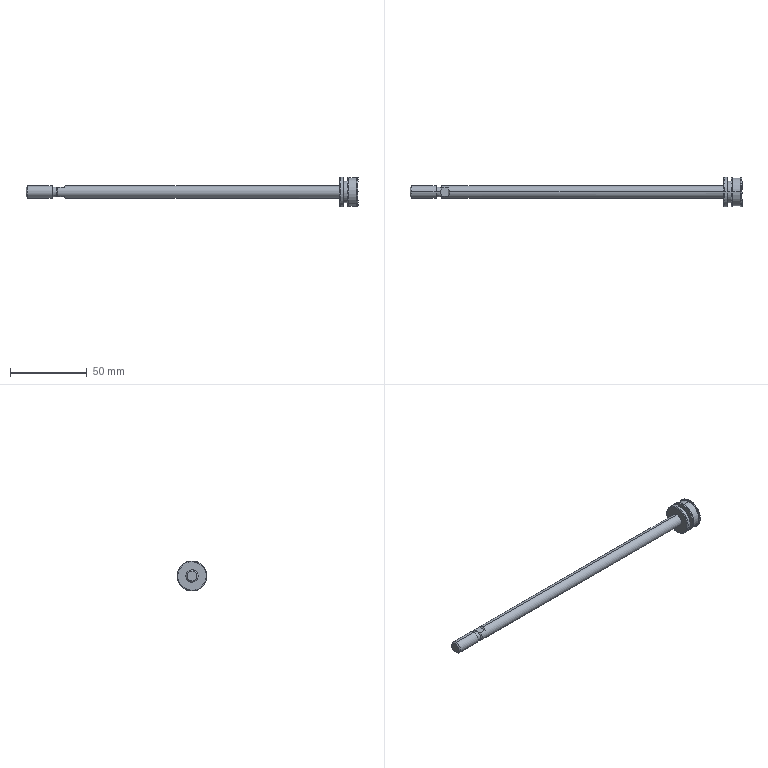Part | STEP file | _MI 20x125-S-U_r | 1 solid | 50 faces | box 216.2 x 19.5 x 19.5 mm | volume 13202 mm3 | cylinder 16 | plane 14 | cone 12 | spline 8 | commonest cylinder face diameters 19.5 x6 8 x4 6.4 x2 14 x2 18.3 x2